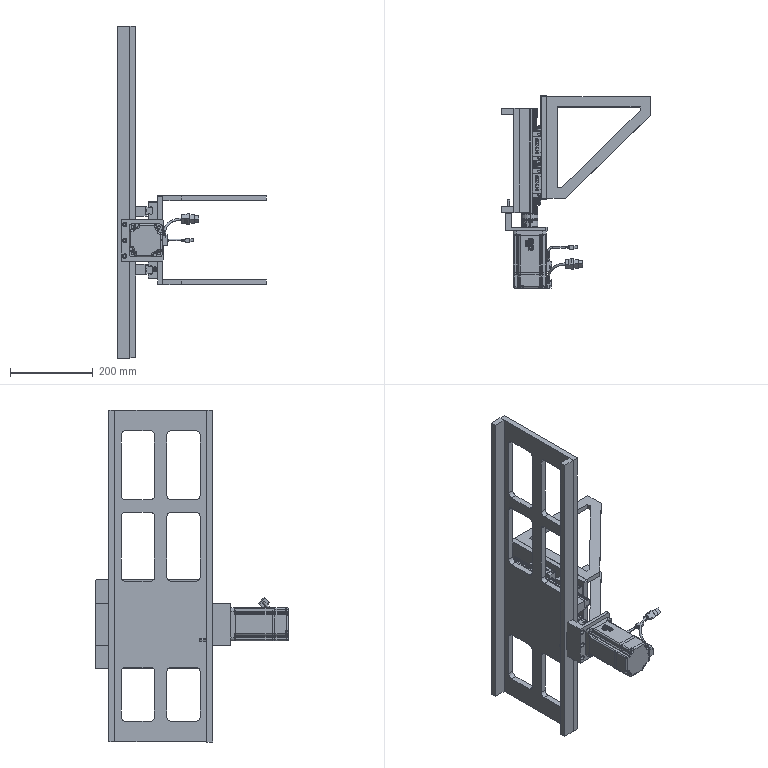Part | SolidWorks | 37 solids | 4043 faces | volume 5456068 mm3 | plane 2302 | cylinder 946 | spline 530 | cone 201 | torus 36 | sphere 28 | commonest cylinder face diameters 1 x71 2 x64 6 x63 5.5 x60 2.6 x48 8 x44